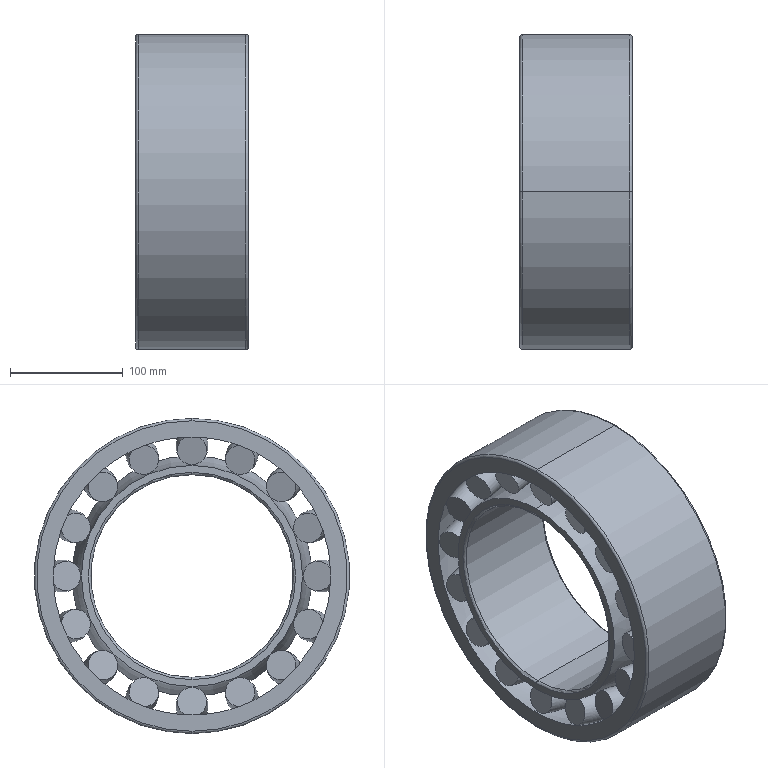Part | SolidWorks | features Revolution 4, Fillet 2, CirPattern 1, MirrorPattern 1, MirrorSolid 1 | 34 solids | 152 faces | box 100 x 280 x 280 mm | volume 2236455 mm3 | torus 76 | plane 68 | cylinder 6 | sphere 2 | commonest cylinder face diameters 180 x2 213.333 x2 280 x2